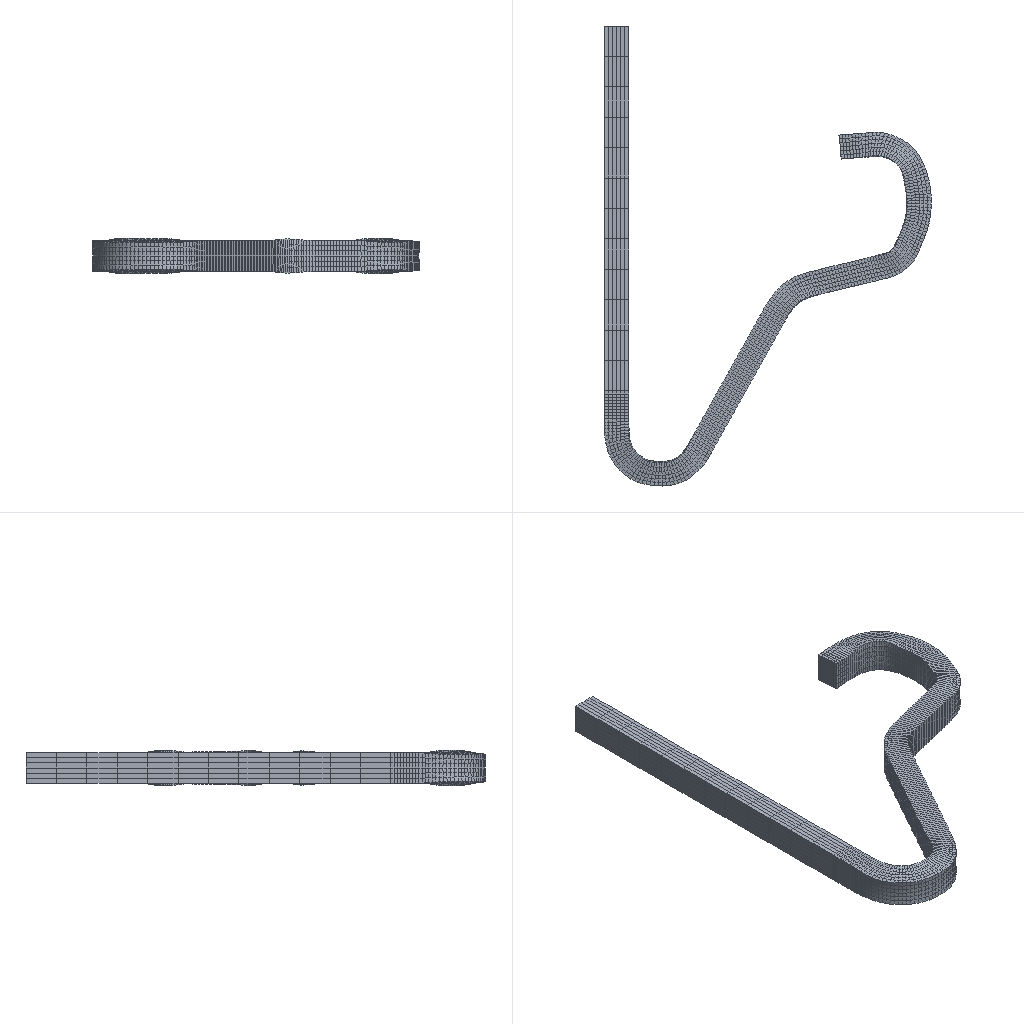Simulation study | abaqus
Set-up summary:
category,name,step,type,value,unit,region
solver,abaqus
solver,version,,,Abaqus/Standard 6.12-3
units,not stated in the deck,,not stated
analysis,deck,,static,static
load_step,Step-1_NF,Step-1_NF,static
load_step,requested,,,1
mesh,nodes,,,10437
mesh,elements,,,7632
element_type,C3D8R,,solid,7632
load,load commands in deck,,count,1
bc,support commands in deck,,count,2
material,C70250,,in results
check,setup vs results,,match,"per instance, exact: element labels, types and connectivity; labels of the nodes the elements use; coordinates of those nodes at SINGLE_PRECISION in 1 of 1 instance(s)"
Abaqus input file, long lists of numbers shortened:
*Heading
** Job name:  Model name: NF
** Generated by: Abaqus/CAE 6.12-3
*Preprint, echo=NO, model=NO, history=NO, contact=NO
**
** PARTS
**
*Part, name=BLANK
*Node
      1,  -27.39,   10.277, -0.125
      2,  -27.39,   10.277, -0.08333
** (10435 more lines like these left out)
*Element, type=C3D8R
   1,    92,    93,   100,    99,     1,     2,     9,     8
   2,    93,    94,   101,   100,     2,     3,    10,     9
** (7630 more lines like these left out)
*Elset, elset=_PickedSet5, internal, generate
    1,  7632,     1
** Section: Section-1
*Solid Section, elset=_PickedSet5, material=C70250
,
*End Part
**
**
** ASSEMBLY
**
*Assembly, name=Assembly
**
*Instance, name=BLANK-1, part=BLANK
*End Instance
**
*Nset, nset=_PickedSet4, internal, instance=BLANK-1
    1,    2,    3,    4,    5,    6,    7,    8,    9,   10,   11,   12,   13,   14,   15,   16
   17,   18,   19,   20,   21,   22,   23,   24,   25,   26,   27,   28,   29,   30,   31,   32
** (9 more lines like these left out)
*Nset, nset=_PickedSet8, internal, instance=BLANK-1
 2385,
*Elset, elset=__PickedSurf9_S2, internal, instance=BLANK-1
 447,
*Surface, type=ELEMENT, name=_PickedSurf9, internal
__PickedSurf9_S2, S2
*Elset, elset=__PickedSurf10_S1, internal, instance=BLANK-1
 425,
*Surface, type=ELEMENT, name=_PickedSurf10, internal
__PickedSurf10_S1, S1
*End Assembly
**
** MATERIALS
**
*Material, name=C70250
*Elastic
131000., 0.341
*Plastic
473.,    0.
816., 0.137
**
** INTERACTION PROPERTIES
**
*Surface Interaction, name=IntProp-1
1.,
*Friction, slip tolerance=0.005
 0.15,
**
** BOUNDARY CONDITIONS
**
** Name: BC-1_Fix Type: Symmetry/Antisymmetry/Encastre
*Boundary
_PickedSet4, ENCASTRE
**
** INTERACTIONS
**
** Interaction: Int-1
*Contact Pair, interaction=IntProp-1, type=SURFACE TO SURFACE
_PickedSurf10, _PickedSurf9
** ----------------------------------------------------------------
**
** STEP: Step-1_NF
**
*Step, name=Step-1_NF, nlgeom=YES
*Static
0.1, 1., 1e-05, 0.1
**
** BOUNDARY CONDITIONS
**
** Name: BC-2_Move Type: Displacement/Rotation
*Boundary
_PickedSet8, 1, 1, -0.5
**
** OUTPUT REQUESTS
**
*Restart, write, frequency=0
**
** FIELD OUTPUT: F-Output-1
**
*Output, field, variable=PRESELECT
**
** HISTORY OUTPUT: H-Output-1
**
*Output, history, variable=PRESELECT
*End Step
Results summary:
result,step,Step-1_NF,partial,increments=10 time=1/1.0
result,analysis,,,static
result,last_loadstep,,,1
result,primary field,,,U
result,reaction total,,FX,-0.0,model units
result,reaction total,,FY,0.0,model units
result,reaction total,,FZ,0.0,model units